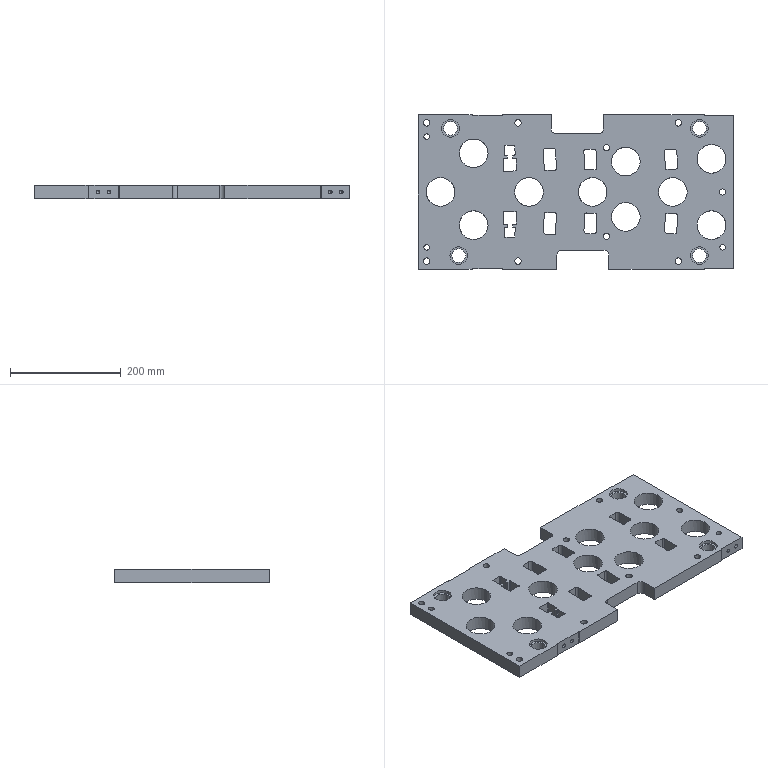Part | NX | features PH-7 2 | 1 solid | 194 faces | box 570 x 280 x 25 mm | volume 3010976 mm3 | cylinder 105 | plane 81 | cone 8 | commonest cylinder face diameters 2 x24 6 x18 18 x13 52.004 x10 10 x9 11.5 x9